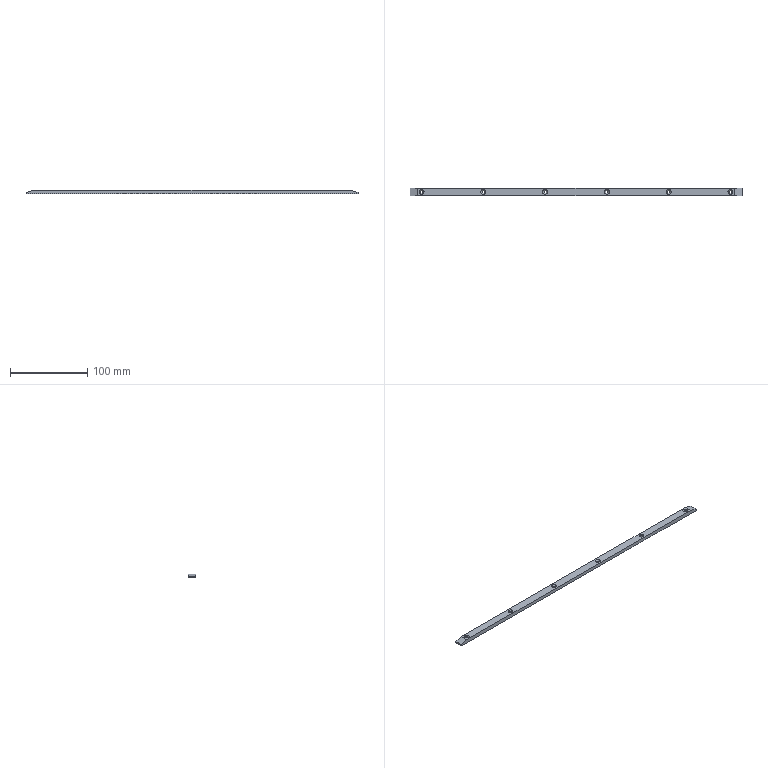Part | NX | features BREP 1 | 1 solid | 32 faces | box 430 x 10 x 5 mm | volume 20841 mm3 | cone 12 | cylinder 12 | plane 8 | commonest cylinder face diameters 3.4 x12
STEP:
#1=CARTESIAN_POINT('',(-203.15,0.,5.));
#2=VERTEX_POINT('',#1);
#3=CARTESIAN_POINT('',(-201.7,0.,3.55));
#4=VERTEX_POINT('',#3);
#5=CARTESIAN_POINT('',(-203.15,0.,5.));
#6=DIRECTION('',(-0.7071,0.,0.7071));
#7=VECTOR('',#6,1000.);
#8=LINE('',#5,#7);
#9=EDGE_CURVE('',#2,#4,#8,.F.);
#10=ORIENTED_EDGE('',*,*,#9,.T.);
#11=CARTESIAN_POINT('',(-198.3,0.,3.55));
#12=VERTEX_POINT('',#11);
#13=CARTESIAN_POINT('',(-200.,0.,3.55));
#14=DIRECTION('',(0.,0.,1.));
#15=DIRECTION('',(1.,0.,0.));
#16=AXIS2_PLACEMENT_3D('',#13,#14,#15);
#17=CIRCLE('',#16,1.7);
#18=EDGE_CURVE('',#12,#4,#17,.T.);
#19=ORIENTED_EDGE('',*,*,#18,.F.);
#20=CARTESIAN_POINT('',(-196.85,0.,5.));
#21=VERTEX_POINT('',#20);
#22=CARTESIAN_POINT('',(-196.85,0.,5.));
#23=DIRECTION('',(0.7071,0.,0.7071));
#24=VECTOR('',#23,1000.);
#25=LINE('',#22,#24);
#26=EDGE_CURVE('',#21,#12,#25,.F.);
#27=ORIENTED_EDGE('',*,*,#26,.F.);
#28=CARTESIAN_POINT('',(-200.,0.,5.));
#29=DIRECTION('',(0.,0.,1.));
#30=DIRECTION('',(1.,0.,0.));
#31=AXIS2_PLACEMENT_3D('',#28,#29,#30);
#32=CIRCLE('',#31,3.15);
#33=EDGE_CURVE('',#21,#2,#32,.T.);
#34=ORIENTED_EDGE('',*,*,#33,.T.);
#35=EDGE_LOOP('',(#10,#19,#27,#34));
#36=FACE_BOUND('',#35,.T.);
#37=CARTESIAN_POINT('',(-200.,0.,5.));
#38=DIRECTION('',(0.,0.,1.));
#39=DIRECTION('',(1.,0.,0.));
#40=AXIS2_PLACEMENT_3D('',#37,#38,#39);
#41=CONICAL_SURFACE('',#40,3.15,0.7854);
#42=ADVANCED_FACE('',(#36),#41,.F.);
#43=CARTESIAN_POINT('',(-201.7,0.,0.));
#44=VERTEX_POINT('',#43);
#45=CARTESIAN_POINT('',(-201.7,0.,5.));
#46=DIRECTION('',(0.,0.,1.));
#47=VECTOR('',#46,1000.);
#48=LINE('',#45,#47);
#49=EDGE_CURVE('',#4,#44,#48,.F.);
#50=ORIENTED_EDGE('',*,*,#49,.T.);
#51=CARTESIAN_POINT('',(-198.3,0.,0.));
#52=VERTEX_POINT('',#51);
#53=CARTESIAN_POINT('',(-200.,0.,0.));
#54=DIRECTION('',(0.,0.,1.));
#55=DIRECTION('',(1.,0.,0.));
#56=AXIS2_PLACEMENT_3D('',#53,#54,#55);
#57=CIRCLE('',#56,1.7);
#58=EDGE_CURVE('',#52,#44,#57,.T.);
#59=ORIENTED_EDGE('',*,*,#58,.F.);
#60=CARTESIAN_POINT('',(-198.3,0.,5.));
#61=DIRECTION('',(0.,0.,1.));
#62=VECTOR('',#61,1000.);
#63=LINE('',#60,#62);
#64=EDGE_CURVE('',#12,#52,#63,.F.);
#65=ORIENTED_EDGE('',*,*,#64,.F.);
#66=ORIENTED_EDGE('',*,*,#18,.T.);
#67=EDGE_LOOP('',(#50,#59,#65,#66));
#68=FACE_BOUND('',#67,.T.);
#69=CARTESIAN_POINT('',(-200.,0.,5.));
#70=DIRECTION('',(0.,0.,1.));
#71=DIRECTION('',(1.,0.,0.));
#72=AXIS2_PLACEMENT_3D('',#69,#70,#71);
#73=CYLINDRICAL_SURFACE('',#72,1.7);
#74=ADVANCED_FACE('',(#68),#73,.F.);
#75=CARTESIAN_POINT('',(-123.15,0.,5.));
#76=VERTEX_POINT('',#75);
#77=CARTESIAN_POINT('',(-121.7,0.,3.55));
#78=VERTEX_POINT('',#77);
#79=CARTESIAN_POINT('',(-123.15,0.,5.));
#80=DIRECTION('',(-0.7071,0.,0.7071));
#81=VECTOR('',#80,1000.);
#82=LINE('',#79,#81);
#83=EDGE_CURVE('',#76,#78,#82,.F.);
#84=ORIENTED_EDGE('',*,*,#83,.T.);
#85=CARTESIAN_POINT('',(-118.3,0.,3.55));
#86=VERTEX_POINT('',#85);
#87=CARTESIAN_POINT('',(-120.,0.,3.55));
#88=DIRECTION('',(0.,0.,1.));
#89=DIRECTION('',(1.,0.,0.));
#90=AXIS2_PLACEMENT_3D('',#87,#88,#89);
#91=CIRCLE('',#90,1.7);
#92=EDGE_CURVE('',#86,#78,#91,.T.);
#93=ORIENTED_EDGE('',*,*,#92,.F.);
#94=CARTESIAN_POINT('',(-116.85,0.,5.));
#95=VERTEX_POINT('',#94);
#96=CARTESIAN_POINT('',(-116.85,0.,5.));
#97=DIRECTION('',(0.7071,0.,0.7071));
#98=VECTOR('',#97,1000.);
#99=LINE('',#96,#98);
#100=EDGE_CURVE('',#95,#86,#99,.F.);
#101=ORIENTED_EDGE('',*,*,#100,.F.);
#102=CARTESIAN_POINT('',(-120.,0.,5.));
#103=DIRECTION('',(0.,0.,1.));
#104=DIRECTION('',(1.,0.,0.));
#105=AXIS2_PLACEMENT_3D('',#102,#103,#104);
#106=CIRCLE('',#105,3.15);
#107=EDGE_CURVE('',#95,#76,#106,.T.);
#108=ORIENTED_EDGE('',*,*,#107,.T.);
#109=EDGE_LOOP('',(#84,#93,#101,#108));
#110=FACE_BOUND('',#109,.T.);
#111=CARTESIAN_POINT('',(-120.,0.,5.));
#112=DIRECTION('',(0.,0.,1.));
#113=DIRECTION('',(1.,0.,0.));
#114=AXIS2_PLACEMENT_3D('',#111,#112,#113);
#115=CONICAL_SURFACE('',#114,3.15,0.7854);
#116=ADVANCED_FACE('',(#110),#115,.F.);
#117=CARTESIAN_POINT('',(-121.7,0.,0.));
#118=VERTEX_POINT('',#117);
#119=CARTESIAN_POINT('',(-121.7,0.,5.));
#120=DIRECTION('',(0.,0.,1.));
#121=VECTOR('',#120,1000.);
#122=LINE('',#119,#121);
#123=EDGE_CURVE('',#78,#118,#122,.F.);
#124=ORIENTED_EDGE('',*,*,#123,.T.);
#125=CARTESIAN_POINT('',(-118.3,0.,0.));
#126=VERTEX_POINT('',#125);
#127=CARTESIAN_POINT('',(-120.,0.,0.));
#128=DIRECTION('',(0.,0.,1.));
#129=DIRECTION('',(1.,0.,0.));
#130=AXIS2_PLACEMENT_3D('',#127,#128,#129);
#131=CIRCLE('',#130,1.7);
#132=EDGE_CURVE('',#126,#118,#131,.T.);
#133=ORIENTED_EDGE('',*,*,#132,.F.);
#134=CARTESIAN_POINT('',(-118.3,0.,5.));
#135=DIRECTION('',(0.,0.,1.));
#136=VECTOR('',#135,1000.);
#137=LINE('',#134,#136);
#138=EDGE_CURVE('',#86,#126,#137,.F.);
#139=ORIENTED_EDGE('',*,*,#138,.F.);
#140=ORIENTED_EDGE('',*,*,#92,.T.);
#141=EDGE_LOOP('',(#124,#133,#139,#140));
#142=FACE_BOUND('',#141,.T.);
#143=CARTESIAN_POINT('',(-120.,0.,5.));
#144=DIRECTION('',(0.,0.,1.));
#145=DIRECTION('',(1.,0.,0.));
#146=AXIS2_PLACEMENT_3D('',#143,#144,#145);
#147=CYLINDRICAL_SURFACE('',#146,1.7);
#148=ADVANCED_FACE('',(#142),#147,.F.);
#149=CARTESIAN_POINT('',(-43.15,0.,5.));
#150=VERTEX_POINT('',#149);
#151=CARTESIAN_POINT('',(-41.7,0.,3.55));
#152=VERTEX_POINT('',#151);
#153=CARTESIAN_POINT('',(-43.15,0.,5.));
#154=DIRECTION('',(-0.7071,0.,0.7071));
#155=VECTOR('',#154,1000.);
#156=LINE('',#153,#155);
#157=EDGE_CURVE('',#150,#152,#156,.F.);
#158=ORIENTED_EDGE('',*,*,#157,.T.);
#159=CARTESIAN_POINT('',(-38.3,0.,3.55));
#160=VERTEX_POINT('',#159);
#161=CARTESIAN_POINT('',(-40.,0.,3.55));
#162=DIRECTION('',(0.,0.,1.));
#163=DIRECTION('',(1.,0.,0.));
#164=AXIS2_PLACEMENT_3D('',#161,#162,#163);
#165=CIRCLE('',#164,1.7);
#166=EDGE_CURVE('',#160,#152,#165,.T.);
#167=ORIENTED_EDGE('',*,*,#166,.F.);
#168=CARTESIAN_POINT('',(-36.85,0.,5.));
#169=VERTEX_POINT('',#168);
#170=CARTESIAN_POINT('',(-36.85,0.,5.));
#171=DIRECTION('',(0.7071,0.,0.7071));
#172=VECTOR('',#171,1000.);
#173=LINE('',#170,#172);
#174=EDGE_CURVE('',#169,#160,#173,.F.);
#175=ORIENTED_EDGE('',*,*,#174,.F.);
#176=CARTESIAN_POINT('',(-40.,0.,5.));
#177=DIRECTION('',(0.,0.,1.));
#178=DIRECTION('',(1.,0.,0.));
#179=AXIS2_PLACEMENT_3D('',#176,#177,#178);
#180=CIRCLE('',#179,3.15);
#181=EDGE_CURVE('',#169,#150,#180,.T.);
#182=ORIENTED_EDGE('',*,*,#181,.T.);
#183=EDGE_LOOP('',(#158,#167,#175,#182));
#184=FACE_BOUND('',#183,.T.);
#185=CARTESIAN_POINT('',(-40.,0.,5.));
#186=DIRECTION('',(0.,0.,1.));
#187=DIRECTION('',(1.,0.,0.));
#188=AXIS2_PLACEMENT_3D('',#185,#186,#187);
#189=CONICAL_SURFACE('',#188,3.15,0.7854);
#190=ADVANCED_FACE('',(#184),#189,.F.);
#191=CARTESIAN_POINT('',(-41.7,0.,0.));
#192=VERTEX_POINT('',#191);
#193=CARTESIAN_POINT('',(-41.7,0.,5.));
#194=DIRECTION('',(0.,0.,1.));
#195=VECTOR('',#194,1000.);
#196=LINE('',#193,#195);
#197=EDGE_CURVE('',#152,#192,#196,.F.);
#198=ORIENTED_EDGE('',*,*,#197,.T.);
#199=CARTESIAN_POINT('',(-38.3,0.,0.));
#200=VERTEX_POINT('',#199);
#201=CARTESIAN_POINT('',(-40.,0.,0.));
#202=DIRECTION('',(0.,0.,1.));
#203=DIRECTION('',(1.,0.,0.));
#204=AXIS2_PLACEMENT_3D('',#201,#202,#203);
#205=CIRCLE('',#204,1.7);
#206=EDGE_CURVE('',#200,#192,#205,.T.);
#207=ORIENTED_EDGE('',*,*,#206,.F.);
#208=CARTESIAN_POINT('',(-38.3,0.,5.));
#209=DIRECTION('',(0.,0.,1.));
#210=VECTOR('',#209,1000.);
#211=LINE('',#208,#210);
#212=EDGE_CURVE('',#160,#200,#211,.F.);
#213=ORIENTED_EDGE('',*,*,#212,.F.);
#214=ORIENTED_EDGE('',*,*,#166,.T.);
#215=EDGE_LOOP('',(#198,#207,#213,#214));
#216=FACE_BOUND('',#215,.T.);
#217=CARTESIAN_POINT('',(-40.,0.,5.));
#218=DIRECTION('',(0.,0.,1.));
#219=DIRECTION('',(1.,0.,0.));
#220=AXIS2_PLACEMENT_3D('',#217,#218,#219);
#221=CYLINDRICAL_SURFACE('',#220,1.7);
#222=ADVANCED_FACE('',(#216),#221,.F.);
#223=CARTESIAN_POINT('',(36.85,0.,5.));
#224=VERTEX_POINT('',#223);
#225=CARTESIAN_POINT('',(38.3,0.,3.55));
#226=VERTEX_POINT('',#225);
#227=CARTESIAN_POINT('',(36.85,0.,5.));
#228=DIRECTION('',(-0.7071,0.,0.7071));
#229=VECTOR('',#228,1000.);
#230=LINE('',#227,#229);
#231=EDGE_CURVE('',#224,#226,#230,.F.);
#232=ORIENTED_EDGE('',*,*,#231,.T.);
#233=CARTESIAN_POINT('',(41.7,0.,3.55));
#234=VERTEX_POINT('',#233);
#235=CARTESIAN_POINT('',(40.,0.,3.55));
#236=DIRECTION('',(0.,0.,1.));
#237=DIRECTION('',(1.,0.,0.));
#238=AXIS2_PLACEMENT_3D('',#235,#236,#237);
#239=CIRCLE('',#238,1.7);
#240=EDGE_CURVE('',#234,#226,#239,.T.);
#241=ORIENTED_EDGE('',*,*,#240,.F.);
#242=CARTESIAN_POINT('',(43.15,0.,5.));
#243=VERTEX_POINT('',#242);
#244=CARTESIAN_POINT('',(43.15,0.,5.));
#245=DIRECTION('',(0.7071,0.,0.7071));
#246=VECTOR('',#245,1000.);
#247=LINE('',#244,#246);
#248=EDGE_CURVE('',#243,#234,#247,.F.);
#249=ORIENTED_EDGE('',*,*,#248,.F.);
#250=CARTESIAN_POINT('',(40.,0.,5.));
#251=DIRECTION('',(0.,0.,1.));
#252=DIRECTION('',(1.,0.,0.));
#253=AXIS2_PLACEMENT_3D('',#250,#251,#252);
#254=CIRCLE('',#253,3.15);
#255=EDGE_CURVE('',#243,#224,#254,.T.);
#256=ORIENTED_EDGE('',*,*,#255,.T.);
#257=EDGE_LOOP('',(#232,#241,#249,#256));
#258=FACE_BOUND('',#257,.T.);
#259=CARTESIAN_POINT('',(40.,0.,5.));
#260=DIRECTION('',(0.,0.,1.));
#261=DIRECTION('',(1.,0.,0.));
#262=AXIS2_PLACEMENT_3D('',#259,#260,#261);
#263=CONICAL_SURFACE('',#262,3.15,0.7854);
#264=ADVANCED_FACE('',(#258),#263,.F.);
#265=CARTESIAN_POINT('',(38.3,0.,0.));
#266=VERTEX_POINT('',#265);
#267=CARTESIAN_POINT('',(38.3,0.,5.));
#268=DIRECTION('',(0.,0.,1.));
#269=VECTOR('',#268,1000.);
#270=LINE('',#267,#269);
#271=EDGE_CURVE('',#226,#266,#270,.F.);
#272=ORIENTED_EDGE('',*,*,#271,.T.);
#273=CARTESIAN_POINT('',(41.7,0.,0.));
#274=VERTEX_POINT('',#273);
#275=CARTESIAN_POINT('',(40.,0.,0.));
#276=DIRECTION('',(0.,0.,1.));
#277=DIRECTION('',(1.,0.,0.));
#278=AXIS2_PLACEMENT_3D('',#275,#276,#277);
#279=CIRCLE('',#278,1.7);
#280=EDGE_CURVE('',#274,#266,#279,.T.);
#281=ORIENTED_EDGE('',*,*,#280,.F.);
#282=CARTESIAN_POINT('',(41.7,0.,5.));
#283=DIRECTION('',(0.,0.,1.));
#284=VECTOR('',#283,1000.);
#285=LINE('',#282,#284);
#286=EDGE_CURVE('',#234,#274,#285,.F.);
#287=ORIENTED_EDGE('',*,*,#286,.F.);
#288=ORIENTED_EDGE('',*,*,#240,.T.);
#289=EDGE_LOOP('',(#272,#281,#287,#288));
#290=FACE_BOUND('',#289,.T.);
#291=CARTESIAN_POINT('',(40.,0.,5.));
#292=DIRECTION('',(0.,0.,1.));
#293=DIRECTION('',(1.,0.,0.));
#294=AXIS2_PLACEMENT_3D('',#291,#292,#293);
#295=CYLINDRICAL_SURFACE('',#294,1.7);
#296=ADVANCED_FACE('',(#290),#295,.F.);
#297=CARTESIAN_POINT('',(116.85,0.,5.));
#298=VERTEX_POINT('',#297);
#299=CARTESIAN_POINT('',(118.3,0.,3.55));
#300=VERTEX_POINT('',#299);
#301=CARTESIAN_POINT('',(116.85,0.,5.));
#302=DIRECTION('',(-0.7071,0.,0.7071));
#303=VECTOR('',#302,1000.);
#304=LINE('',#301,#303);
#305=EDGE_CURVE('',#298,#300,#304,.F.);
#306=ORIENTED_EDGE('',*,*,#305,.T.);
#307=CARTESIAN_POINT('',(121.7,0.,3.55));
#308=VERTEX_POINT('',#307);
#309=CARTESIAN_POINT('',(120.,0.,3.55));
#310=DIRECTION('',(0.,0.,1.));
#311=DIRECTION('',(1.,0.,0.));
#312=AXIS2_PLACEMENT_3D('',#309,#310,#311);
#313=CIRCLE('',#312,1.7);
#314=EDGE_CURVE('',#308,#300,#313,.T.);
#315=ORIENTED_EDGE('',*,*,#314,.F.);
#316=CARTESIAN_POINT('',(123.15,0.,5.));
#317=VERTEX_POINT('',#316);
#318=CARTESIAN_POINT('',(123.15,0.,5.));
#319=DIRECTION('',(0.7071,0.,0.7071));
#320=VECTOR('',#319,1000.);
#321=LINE('',#318,#320);
#322=EDGE_CURVE('',#317,#308,#321,.F.);
#323=ORIENTED_EDGE('',*,*,#322,.F.);
#324=CARTESIAN_POINT('',(120.,0.,5.));
#325=DIRECTION('',(0.,0.,1.));
#326=DIRECTION('',(1.,0.,0.));
#327=AXIS2_PLACEMENT_3D('',#324,#325,#326);
#328=CIRCLE('',#327,3.15);
#329=EDGE_CURVE('',#317,#298,#328,.T.);
#330=ORIENTED_EDGE('',*,*,#329,.T.);
#331=EDGE_LOOP('',(#306,#315,#323,#330));
#332=FACE_BOUND('',#331,.T.);
#333=CARTESIAN_POINT('',(120.,0.,5.));
#334=DIRECTION('',(0.,0.,1.));
#335=DIRECTION('',(1.,0.,0.));
#336=AXIS2_PLACEMENT_3D('',#333,#334,#335);
#337=CONICAL_SURFACE('',#336,3.15,0.7854);
#338=ADVANCED_FACE('',(#332),#337,.F.);
#339=CARTESIAN_POINT('',(118.3,0.,0.));
#340=VERTEX_POINT('',#339);
#341=CARTESIAN_POINT('',(118.3,0.,5.));
#342=DIRECTION('',(0.,0.,1.));
#343=VECTOR('',#342,1000.);
#344=LINE('',#341,#343);
#345=EDGE_CURVE('',#300,#340,#344,.F.);
#346=ORIENTED_EDGE('',*,*,#345,.T.);
#347=CARTESIAN_POINT('',(121.7,0.,0.));
#348=VERTEX_POINT('',#347);
#349=CARTESIAN_POINT('',(120.,0.,0.));
#350=DIRECTION('',(0.,0.,1.));
#351=DIRECTION('',(1.,0.,0.));
#352=AXIS2_PLACEMENT_3D('',#349,#350,#351);
#353=CIRCLE('',#352,1.7);
#354=EDGE_CURVE('',#348,#340,#353,.T.);
#355=ORIENTED_EDGE('',*,*,#354,.F.);
#356=CARTESIAN_POINT('',(121.7,0.,5.));
#357=DIRECTION('',(0.,0.,1.));
#358=VECTOR('',#357,1000.);
#359=LINE('',#356,#358);
#360=EDGE_CURVE('',#308,#348,#359,.F.);
#361=ORIENTED_EDGE('',*,*,#360,.F.);
#362=ORIENTED_EDGE('',*,*,#314,.T.);
#363=EDGE_LOOP('',(#346,#355,#361,#362));
#364=FACE_BOUND('',#363,.T.);
#365=CARTESIAN_POINT('',(120.,0.,5.));
#366=DIRECTION('',(0.,0.,1.));
#367=DIRECTION('',(1.,0.,0.));
#368=AXIS2_PLACEMENT_3D('',#365,#366,#367);
#369=CYLINDRICAL_SURFACE('',#368,1.7);
#370=ADVANCED_FACE('',(#364),#369,.F.);
#371=CARTESIAN_POINT('',(196.85,0.,5.));
#372=VERTEX_POINT('',#371);
#373=CARTESIAN_POINT('',(198.3,0.,3.55));
#374=VERTEX_POINT('',#373);
#375=CARTESIAN_POINT('',(196.85,0.,5.));
#376=DIRECTION('',(-0.7071,0.,0.7071));
#377=VECTOR('',#376,1000.);
#378=LINE('',#375,#377);
#379=EDGE_CURVE('',#372,#374,#378,.F.);
#380=ORIENTED_EDGE('',*,*,#379,.T.);
#381=CARTESIAN_POINT('',(201.7,0.,3.55));
#382=VERTEX_POINT('',#381);
#383=CARTESIAN_POINT('',(200.,0.,3.55));
#384=DIRECTION('',(0.,0.,1.));
#385=DIRECTION('',(1.,0.,0.));
#386=AXIS2_PLACEMENT_3D('',#383,#384,#385);
#387=CIRCLE('',#386,1.7);
#388=EDGE_CURVE('',#382,#374,#387,.T.);
#389=ORIENTED_EDGE('',*,*,#388,.F.);
#390=CARTESIAN_POINT('',(203.15,0.,5.));
#391=VERTEX_POINT('',#390);
#392=CARTESIAN_POINT('',(203.15,0.,5.));
#393=DIRECTION('',(0.7071,0.,0.7071));
#394=VECTOR('',#393,1000.);
#395=LINE('',#392,#394);
#396=EDGE_CURVE('',#391,#382,#395,.F.);
#397=ORIENTED_EDGE('',*,*,#396,.F.);
#398=CARTESIAN_POINT('',(200.,0.,5.));
#399=DIRECTION('',(0.,0.,1.));
#400=DIRECTION('',(1.,0.,0.));
#401=AXIS2_PLACEMENT_3D('',#398,#399,#400);
#402=CIRCLE('',#401,3.15);
#403=EDGE_CURVE('',#391,#372,#402,.T.);
#404=ORIENTED_EDGE('',*,*,#403,.T.);
#405=EDGE_LOOP('',(#380,#389,#397,#404));
#406=FACE_BOUND('',#405,.T.);
#407=CARTESIAN_POINT('',(200.,0.,5.));
#408=DIRECTION('',(0.,0.,1.));
#409=DIRECTION('',(1.,0.,0.));
#410=AXIS2_PLACEMENT_3D('',#407,#408,#409);
#411=CONICAL_SURFACE('',#410,3.15,0.7854);
#412=ADVANCED_FACE('',(#406),#411,.F.);
#413=CARTESIAN_POINT('',(198.3,0.,0.));
#414=VERTEX_POINT('',#413);
#415=CARTESIAN_POINT('',(198.3,0.,5.));
#416=DIRECTION('',(0.,0.,1.));
#417=VECTOR('',#416,1000.);
#418=LINE('',#415,#417);
#419=EDGE_CURVE('',#374,#414,#418,.F.);
#420=ORIENTED_EDGE('',*,*,#419,.T.);
#421=CARTESIAN_POINT('',(201.7,0.,0.));
#422=VERTEX_POINT('',#421);
#423=CARTESIAN_POINT('',(200.,0.,0.));
#424=DIRECTION('',(0.,0.,1.));
#425=DIRECTION('',(1.,0.,0.));
#426=AXIS2_PLACEMENT_3D('',#423,#424,#425);
#427=CIRCLE('',#426,1.7);
#428=EDGE_CURVE('',#422,#414,#427,.T.);
#429=ORIENTED_EDGE('',*,*,#428,.F.);
#430=CARTESIAN_POINT('',(201.7,0.,5.));
#431=DIRECTION('',(0.,0.,1.));
#432=VECTOR('',#431,1000.);
#433=LINE('',#430,#432);
#434=EDGE_CURVE('',#382,#422,#433,.F.);
#435=ORIENTED_EDGE('',*,*,#434,.F.);
#436=ORIENTED_EDGE('',*,*,#388,.T.);
#437=EDGE_LOOP('',(#420,#429,#435,#436));
#438=FACE_BOUND('',#437,.T.);
#439=CARTESIAN_POINT('',(200.,0.,5.));
#440=DIRECTION('',(0.,0.,1.));
#441=DIRECTION('',(1.,0.,0.));
#442=AXIS2_PLACEMENT_3D('',#439,#440,#441);
#443=CYLINDRICAL_SURFACE('',#442,1.7);
#444=ADVANCED_FACE('',(#438),#443,.F.);
#445=CARTESIAN_POINT('',(-215.,5.,2.));
#446=VERTEX_POINT('',#445);
#447=CARTESIAN_POINT('',(-205.,5.,5.));
#448=VERTEX_POINT('',#447);
#449=CARTESIAN_POINT('',(-205.,5.,5.));
#450=DIRECTION('',(0.9578,0.,0.2873));
#451=VECTOR('',#450,1000.);
#452=LINE('',#449,#451);
#453=EDGE_CURVE('',#446,#448,#452,.T.);
#454=ORIENTED_EDGE('',*,*,#453,.F.);
#455=CARTESIAN_POINT('',(-215.,-5.,2.));
#456=VERTEX_POINT('',#455);
#457=CARTESIAN_POINT('',(-215.,-5.,2.));
#458=DIRECTION('',(0.,1.,0.));
#459=VECTOR('',#458,1000.);
#460=LINE('',#457,#459);
#461=EDGE_CURVE('',#456,#446,#460,.T.);
#462=ORIENTED_EDGE('',*,*,#461,.F.);
#463=CARTESIAN_POINT('',(-205.,-5.,5.));
#464=VERTEX_POINT('',#463);
#465=CARTESIAN_POINT('',(-205.,-5.,5.));
#466=DIRECTION('',(-0.9578,0.,-0.2873));
#467=VECTOR('',#466,1000.);
#468=LINE('',#465,#467);
#469=EDGE_CURVE('',#464,#456,#468,.T.);
#470=ORIENTED_EDGE('',*,*,#469,.F.);
#471=CARTESIAN_POINT('',(-205.,0.,5.));
#472=DIRECTION('',(0.,-1.,0.));
#473=VECTOR('',#472,1000.);
#474=LINE('',#471,#473);
#475=EDGE_CURVE('',#448,#464,#474,.T.);
#476=ORIENTED_EDGE('',*,*,#475,.F.);
#477=EDGE_LOOP('',(#454,#462,#470,#476));
#478=FACE_BOUND('',#477,.T.);
#479=CARTESIAN_POINT('',(-205.,0.,5.));
#480=DIRECTION('',(0.2873,0.,-0.9578));
#481=DIRECTION('',(0.,-1.,0.));
#482=AXIS2_PLACEMENT_3D('',#479,#480,#481);
#483=PLANE('',#482);
#484=ADVANCED_FACE('',(#478),#483,.F.);
#485=CARTESIAN_POINT('',(215.,-5.,2.));
#486=VERTEX_POINT('',#485);
#487=CARTESIAN_POINT('',(205.,-5.,5.));
#488=VERTEX_POINT('',#487);
#489=CARTESIAN_POINT('',(205.,-5.,5.));
#490=DIRECTION('',(-0.9578,0.,0.2873));
#491=VECTOR('',#490,1000.);
#492=LINE('',#489,#491);
#493=EDGE_CURVE('',#486,#488,#492,.T.);
#494=ORIENTED_EDGE('',*,*,#493,.F.);
#495=CARTESIAN_POINT('',(215.,5.,2.));
#496=VERTEX_POINT('',#495);
#497=CARTESIAN_POINT('',(215.,-5.,2.));
#498=DIRECTION('',(0.,-1.,0.));
#499=VECTOR('',#498,1000.);
#500=LINE('',#497,#499);
#501=EDGE_CURVE('',#496,#486,#500,.T.);
#502=ORIENTED_EDGE('',*,*,#501,.F.);
#503=CARTESIAN_POINT('',(205.,5.,5.));
#504=VERTEX_POINT('',#503);
#505=CARTESIAN_POINT('',(205.,5.,5.));
#506=DIRECTION('',(0.9578,0.,-0.2873));
#507=VECTOR('',#506,1000.);
#508=LINE('',#505,#507);
#509=EDGE_CURVE('',#504,#496,#508,.T.);
#510=ORIENTED_EDGE('',*,*,#509,.F.);
#511=CARTESIAN_POINT('',(205.,0.,5.));
#512=DIRECTION('',(0.,1.,0.));
#513=VECTOR('',#512,1000.);
#514=LINE('',#511,#513);
#515=EDGE_CURVE('',#488,#504,#514,.T.);
#516=ORIENTED_EDGE('',*,*,#515,.F.);
#517=EDGE_LOOP('',(#494,#502,#510,#516));
#518=FACE_BOUND('',#517,.T.);
#519=CARTESIAN_POINT('',(205.,0.,5.));
#520=DIRECTION('',(-0.2873,0.,-0.9578));
#521=DIRECTION('',(0.,1.,0.));
#522=AXIS2_PLACEMENT_3D('',#519,#520,#521);
#523=PLANE('',#522);
#524=ADVANCED_FACE('',(#518),#523,.F.);
#525=CARTESIAN_POINT('',(215.,-5.,0.));
#526=VERTEX_POINT('',#525);
#527=CARTESIAN_POINT('',(215.,5.,0.));
#528=VERTEX_POINT('',#527);
#529=CARTESIAN_POINT('',(215.,-5.,0.));
#530=DIRECTION('',(0.,1.,0.));
#531=VECTOR('',#530,1000.);
#532=LINE('',#529,#531);
#533=EDGE_CURVE('',#526,#528,#532,.T.);
#534=ORIENTED_EDGE('',*,*,#533,.F.);
#535=CARTESIAN_POINT('',(-215.,-5.,0.));
#536=VERTEX_POINT('',#535);
#537=CARTESIAN_POINT('',(-215.,-5.,0.));
#538=DIRECTION('',(1.,0.,0.));
#539=VECTOR('',#538,1000.);
#540=LINE('',#537,#539);
#541=EDGE_CURVE('',#536,#526,#540,.T.);
#542=ORIENTED_EDGE('',*,*,#541,.F.);
#543=CARTESIAN_POINT('',(-215.,5.,0.));
#544=VERTEX_POINT('',#543);
#545=CARTESIAN_POINT('',(-215.,-5.,0.));
#546=DIRECTION('',(0.,-1.,0.));
#547=VECTOR('',#546,1000.);
#548=LINE('',#545,#547);
#549=EDGE_CURVE('',#544,#536,#548,.T.);
#550=ORIENTED_EDGE('',*,*,#549,.F.);
#551=CARTESIAN_POINT('',(-215.,5.,0.));
#552=DIRECTION('',(-1.,0.,0.));
#553=VECTOR('',#552,1000.);
#554=LINE('',#551,#553);
#555=EDGE_CURVE('',#528,#544,#554,.T.);
#556=ORIENTED_EDGE('',*,*,#555,.F.);
#557=EDGE_LOOP('',(#534,#542,#550,#556));
#558=FACE_BOUND('',#557,.T.);
#559=ORIENTED_EDGE('',*,*,#428,.T.);
#560=CARTESIAN_POINT('',(200.,0.,0.));
#561=DIRECTION('',(0.,0.,1.));
#562=DIRECTION('',(1.,0.,0.));
#563=AXIS2_PLACEMENT_3D('',#560,#561,#562);
#564=CIRCLE('',#563,1.7);
#565=EDGE_CURVE('',#414,#422,#564,.T.);
#566=ORIENTED_EDGE('',*,*,#565,.T.);
#567=EDGE_LOOP('',(#559,#566));
#568=FACE_BOUND('',#567,.T.);
#569=ORIENTED_EDGE('',*,*,#354,.T.);
#570=CARTESIAN_POINT('',(120.,0.,0.));
#571=DIRECTION('',(0.,0.,1.));
#572=DIRECTION('',(1.,0.,0.));
#573=AXIS2_PLACEMENT_3D('',#570,#571,#572);
#574=CIRCLE('',#573,1.7);
#575=EDGE_CURVE('',#340,#348,#574,.T.);
#576=ORIENTED_EDGE('',*,*,#575,.T.);
#577=EDGE_LOOP('',(#569,#576));
#578=FACE_BOUND('',#577,.T.);
#579=ORIENTED_EDGE('',*,*,#280,.T.);
#580=CARTESIAN_POINT('',(40.,0.,0.));
#581=DIRECTION('',(0.,0.,1.));
#582=DIRECTION('',(1.,0.,0.));
#583=AXIS2_PLACEMENT_3D('',#580,#581,#582);
#584=CIRCLE('',#583,1.7);
#585=EDGE_CURVE('',#266,#274,#584,.T.);
#586=ORIENTED_EDGE('',*,*,#585,.T.);
#587=EDGE_LOOP('',(#579,#586));
#588=FACE_BOUND('',#587,.T.);
#589=ORIENTED_EDGE('',*,*,#206,.T.);
#590=CARTESIAN_POINT('',(-40.,0.,0.));
#591=DIRECTION('',(0.,0.,1.));
#592=DIRECTION('',(1.,0.,0.));
#593=AXIS2_PLACEMENT_3D('',#590,#591,#592);
#594=CIRCLE('',#593,1.7);
#595=EDGE_CURVE('',#192,#200,#594,.T.);
#596=ORIENTED_EDGE('',*,*,#595,.T.);
#597=EDGE_LOOP('',(#589,#596));
#598=FACE_BOUND('',#597,.T.);
#599=ORIENTED_EDGE('',*,*,#132,.T.);
#600=CARTESIAN_POINT('',(-120.,0.,0.));
#601=DIRECTION('',(0.,0.,1.));
#602=DIRECTION('',(1.,0.,0.));
#603=AXIS2_PLACEMENT_3D('',#600,#601,#602);
#604=CIRCLE('',#603,1.7);
#605=EDGE_CURVE('',#118,#126,#604,.T.);
#606=ORIENTED_EDGE('',*,*,#605,.T.);
#607=EDGE_LOOP('',(#599,#606));
#608=FACE_BOUND('',#607,.T.);
#609=ORIENTED_EDGE('',*,*,#58,.T.);
#610=CARTESIAN_POINT('',(-200.,0.,0.));
#611=DIRECTION('',(0.,0.,1.));
#612=DIRECTION('',(1.,0.,0.));
#613=AXIS2_PLACEMENT_3D('',#610,#611,#612);
#614=CIRCLE('',#613,1.7);
#615=EDGE_CURVE('',#44,#52,#614,.T.);
#616=ORIENTED_EDGE('',*,*,#615,.T.);
#617=EDGE_LOOP('',(#609,#616));
#618=FACE_BOUND('',#617,.T.);
#619=CARTESIAN_POINT('',(0.,0.,0.));
#620=DIRECTION('',(0.,0.,-1.));
#621=DIRECTION('',(-1.,0.,0.));
#622=AXIS2_PLACEMENT_3D('',#619,#620,#621);
#623=PLANE('',#622);
#624=ADVANCED_FACE('',(#558,#568,#578,#588,#598,#608,#618),#623,.T.);
#625=CARTESIAN_POINT('',(215.,-5.,5.));
#626=DIRECTION('',(0.,0.,-1.));
#627=VECTOR('',#626,1000.);
#628=LINE('',#625,#627);
#629=EDGE_CURVE('',#486,#526,#628,.T.);
#630=ORIENTED_EDGE('',*,*,#629,.F.);
#631=ORIENTED_EDGE('',*,*,#493,.T.);
#632=CARTESIAN_POINT('',(-215.,-5.,5.));
#633=DIRECTION('',(1.,0.,0.));
#634=VECTOR('',#633,1000.);
#635=LINE('',#632,#634);
#636=EDGE_CURVE('',#464,#488,#635,.T.);
#637=ORIENTED_EDGE('',*,*,#636,.F.);
#638=ORIENTED_EDGE('',*,*,#469,.T.);
#639=CARTESIAN_POINT('',(-215.,-5.,5.));
#640=DIRECTION('',(0.,0.,-1.));
#641=VECTOR('',#640,1000.);
#642=LINE('',#639,#641);
#643=EDGE_CURVE('',#456,#536,#642,.T.);
#644=ORIENTED_EDGE('',*,*,#643,.T.);
#645=ORIENTED_EDGE('',*,*,#541,.T.);
#646=EDGE_LOOP('',(#630,#631,#637,#638,#644,#645));
#647=FACE_BOUND('',#646,.T.);
#648=CARTESIAN_POINT('',(-215.,-5.,5.));
#649=DIRECTION('',(0.,1.,0.));
#650=DIRECTION('',(0.,0.,1.));
#651=AXIS2_PLACEMENT_3D('',#648,#649,#650);
#652=PLANE('',#651);
#653=ADVANCED_FACE('',(#647),#652,.F.);
#654=ORIENTED_EDGE('',*,*,#643,.F.);
#655=ORIENTED_EDGE('',*,*,#461,.T.);
#656=CARTESIAN_POINT('',(-215.,5.,5.));
#657=DIRECTION('',(0.,0.,-1.));
#658=VECTOR('',#657,1000.);
#659=LINE('',#656,#658);
#660=EDGE_CURVE('',#446,#544,#659,.T.);
#661=ORIENTED_EDGE('',*,*,#660,.T.);
#662=ORIENTED_EDGE('',*,*,#549,.T.);
#663=EDGE_LOOP('',(#654,#655,#661,#662));
#664=FACE_BOUND('',#663,.T.);
#665=CARTESIAN_POINT('',(-215.,-5.,5.));
#666=DIRECTION('',(1.,0.,0.));
#667=DIRECTION('',(0.,0.,-1.));
#668=AXIS2_PLACEMENT_3D('',#665,#666,#667);
#669=PLANE('',#668);
#670=ADVANCED_FACE('',(#664),#669,.F.);
#671=CARTESIAN_POINT('',(-215.,5.,5.));
#672=DIRECTION('',(-1.,0.,0.));
#673=VECTOR('',#672,1000.);
#674=LINE('',#671,#673);
#675=EDGE_CURVE('',#504,#448,#674,.T.);
#676=ORIENTED_EDGE('',*,*,#675,.F.);
#677=ORIENTED_EDGE('',*,*,#509,.T.);
#678=CARTESIAN_POINT('',(215.,5.,5.));
#679=DIRECTION('',(0.,0.,-1.));
#680=VECTOR('',#679,1000.);
#681=LINE('',#678,#680);
#682=EDGE_CURVE('',#496,#528,#681,.T.);
#683=ORIENTED_EDGE('',*,*,#682,.T.);
#684=ORIENTED_EDGE('',*,*,#555,.T.);
#685=ORIENTED_EDGE('',*,*,#660,.F.);
#686=ORIENTED_EDGE('',*,*,#453,.T.);
#687=EDGE_LOOP('',(#676,#677,#683,#684,#685,#686));
#688=FACE_BOUND('',#687,.T.);
#689=CARTESIAN_POINT('',(-215.,5.,5.));
#690=DIRECTION('',(0.,-1.,0.));
#691=DIRECTION('',(0.,0.,-1.));
#692=AXIS2_PLACEMENT_3D('',#689,#690,#691);
#693=PLANE('',#692);
#694=ADVANCED_FACE('',(#688),#693,.F.);
#695=ORIENTED_EDGE('',*,*,#682,.F.);
#696=ORIENTED_EDGE('',*,*,#501,.T.);
#697=ORIENTED_EDGE('',*,*,#629,.T.);
#698=ORIENTED_EDGE('',*,*,#533,.T.);
#699=EDGE_LOOP('',(#695,#696,#697,#698));
#700=FACE_BOUND('',#699,.T.);
#701=CARTESIAN_POINT('',(215.,-5.,5.));
#702=DIRECTION('',(-1.,0.,0.));
#703=DIRECTION('',(0.,0.,1.));
#704=AXIS2_PLACEMENT_3D('',#701,#702,#703);
#705=PLANE('',#704);
#706=ADVANCED_FACE('',(#700),#705,.F.);
#707=ORIENTED_EDGE('',*,*,#255,.F.);
#708=CARTESIAN_POINT('',(40.,0.,5.));
#709=DIRECTION('',(0.,0.,1.));
#710=DIRECTION('',(1.,0.,0.));
#711=AXIS2_PLACEMENT_3D('',#708,#709,#710);
#712=CIRCLE('',#711,3.15);
#713=EDGE_CURVE('',#224,#243,#712,.T.);
#714=ORIENTED_EDGE('',*,*,#713,.F.);
#715=EDGE_LOOP('',(#707,#714));
#716=FACE_BOUND('',#715,.T.);
#717=ORIENTED_EDGE('',*,*,#636,.T.);
#718=ORIENTED_EDGE('',*,*,#515,.T.);
#719=ORIENTED_EDGE('',*,*,#675,.T.);
#720=ORIENTED_EDGE('',*,*,#475,.T.);
#721=EDGE_LOOP('',(#717,#718,#719,#720));
#722=FACE_BOUND('',#721,.T.);
#723=ORIENTED_EDGE('',*,*,#403,.F.);
#724=CARTESIAN_POINT('',(200.,0.,5.));
#725=DIRECTION('',(0.,0.,1.));
#726=DIRECTION('',(1.,0.,0.));
#727=AXIS2_PLACEMENT_3D('',#724,#725,#726);
#728=CIRCLE('',#727,3.15);
#729=EDGE_CURVE('',#372,#391,#728,.T.);
#730=ORIENTED_EDGE('',*,*,#729,.F.);
#731=EDGE_LOOP('',(#723,#730));
#732=FACE_BOUND('',#731,.T.);
#733=ORIENTED_EDGE('',*,*,#329,.F.);
#734=CARTESIAN_POINT('',(120.,0.,5.));
#735=DIRECTION('',(0.,0.,1.));
#736=DIRECTION('',(1.,0.,0.));
#737=AXIS2_PLACEMENT_3D('',#734,#735,#736);
#738=CIRCLE('',#737,3.15);
#739=EDGE_CURVE('',#298,#317,#738,.T.);
#740=ORIENTED_EDGE('',*,*,#739,.F.);
#741=EDGE_LOOP('',(#733,#740));
#742=FACE_BOUND('',#741,.T.);
#743=ORIENTED_EDGE('',*,*,#181,.F.);
#744=CARTESIAN_POINT('',(-40.,0.,5.));
#745=DIRECTION('',(0.,0.,1.));
#746=DIRECTION('',(1.,0.,0.));
#747=AXIS2_PLACEMENT_3D('',#744,#745,#746);
#748=CIRCLE('',#747,3.15);
#749=EDGE_CURVE('',#150,#169,#748,.T.);
#750=ORIENTED_EDGE('',*,*,#749,.F.);
#751=EDGE_LOOP('',(#743,#750));
#752=FACE_BOUND('',#751,.T.);
#753=ORIENTED_EDGE('',*,*,#107,.F.);
#754=CARTESIAN_POINT('',(-120.,0.,5.));
#755=DIRECTION('',(0.,0.,1.));
#756=DIRECTION('',(1.,0.,0.));
#757=AXIS2_PLACEMENT_3D('',#754,#755,#756);
#758=CIRCLE('',#757,3.15);
#759=EDGE_CURVE('',#76,#95,#758,.T.);
#760=ORIENTED_EDGE('',*,*,#759,.F.);
#761=EDGE_LOOP('',(#753,#760));
#762=FACE_BOUND('',#761,.T.);
#763=ORIENTED_EDGE('',*,*,#33,.F.);
#764=CARTESIAN_POINT('',(-200.,0.,5.));
#765=DIRECTION('',(0.,0.,1.));
#766=DIRECTION('',(1.,0.,0.));
#767=AXIS2_PLACEMENT_3D('',#764,#765,#766);
#768=CIRCLE('',#767,3.15);
#769=EDGE_CURVE('',#2,#21,#768,.T.);
#770=ORIENTED_EDGE('',*,*,#769,.F.);
#771=EDGE_LOOP('',(#763,#770));
#772=FACE_BOUND('',#771,.T.);
#773=CARTESIAN_POINT('',(0.,0.,5.));
#774=DIRECTION('',(0.,0.,-1.));
#775=DIRECTION('',(-1.,0.,0.));
#776=AXIS2_PLACEMENT_3D('',#773,#774,#775);
#777=PLANE('',#776);
#778=ADVANCED_FACE('',(#716,#722,#732,#742,#752,#762,#772),#777,.F.);
#779=ORIENTED_EDGE('',*,*,#565,.F.);
#780=ORIENTED_EDGE('',*,*,#419,.F.);
#781=CARTESIAN_POINT('',(200.,0.,3.55));
#782=DIRECTION('',(0.,0.,1.));
#783=DIRECTION('',(1.,0.,0.));
#784=AXIS2_PLACEMENT_3D('',#781,#782,#783);
#785=CIRCLE('',#784,1.7);
#786=EDGE_CURVE('',#374,#382,#785,.T.);
#787=ORIENTED_EDGE('',*,*,#786,.T.);
#788=ORIENTED_EDGE('',*,*,#434,.T.);
#789=EDGE_LOOP('',(#779,#780,#787,#788));
#790=FACE_BOUND('',#789,.T.);
#791=CARTESIAN_POINT('',(200.,0.,5.));
#792=DIRECTION('',(0.,0.,1.));
#793=DIRECTION('',(1.,0.,0.));
#794=AXIS2_PLACEMENT_3D('',#791,#792,#793);
#795=CYLINDRICAL_SURFACE('',#794,1.7);
#796=ADVANCED_FACE('',(#790),#795,.F.);
#797=ORIENTED_EDGE('',*,*,#786,.F.);
#798=ORIENTED_EDGE('',*,*,#379,.F.);
#799=ORIENTED_EDGE('',*,*,#729,.T.);
#800=ORIENTED_EDGE('',*,*,#396,.T.);
#801=EDGE_LOOP('',(#797,#798,#799,#800));
#802=FACE_BOUND('',#801,.T.);
#803=CARTESIAN_POINT('',(200.,0.,5.));
#804=DIRECTION('',(0.,0.,1.));
#805=DIRECTION('',(1.,0.,0.));
#806=AXIS2_PLACEMENT_3D('',#803,#804,#805);
#807=CONICAL_SURFACE('',#806,3.15,0.7854);
#808=ADVANCED_FACE('',(#802),#807,.F.);
#809=ORIENTED_EDGE('',*,*,#575,.F.);
#810=ORIENTED_EDGE('',*,*,#345,.F.);
#811=CARTESIAN_POINT('',(120.,0.,3.55));
#812=DIRECTION('',(0.,0.,1.));
#813=DIRECTION('',(1.,0.,0.));
#814=AXIS2_PLACEMENT_3D('',#811,#812,#813);
#815=CIRCLE('',#814,1.7);
#816=EDGE_CURVE('',#300,#308,#815,.T.);
#817=ORIENTED_EDGE('',*,*,#816,.T.);
#818=ORIENTED_EDGE('',*,*,#360,.T.);
#819=EDGE_LOOP('',(#809,#810,#817,#818));
#820=FACE_BOUND('',#819,.T.);
#821=CARTESIAN_POINT('',(120.,0.,5.));
#822=DIRECTION('',(0.,0.,1.));
#823=DIRECTION('',(1.,0.,0.));
#824=AXIS2_PLACEMENT_3D('',#821,#822,#823);
#825=CYLINDRICAL_SURFACE('',#824,1.7);
#826=ADVANCED_FACE('',(#820),#825,.F.);
#827=ORIENTED_EDGE('',*,*,#816,.F.);
#828=ORIENTED_EDGE('',*,*,#305,.F.);
#829=ORIENTED_EDGE('',*,*,#739,.T.);
#830=ORIENTED_EDGE('',*,*,#322,.T.);
#831=EDGE_LOOP('',(#827,#828,#829,#830));
#832=FACE_BOUND('',#831,.T.);
#833=CARTESIAN_POINT('',(120.,0.,5.));
#834=DIRECTION('',(0.,0.,1.));
#835=DIRECTION('',(1.,0.,0.));
#836=AXIS2_PLACEMENT_3D('',#833,#834,#835);
#837=CONICAL_SURFACE('',#836,3.15,0.7854);
#838=ADVANCED_FACE('',(#832),#837,.F.);
#839=ORIENTED_EDGE('',*,*,#585,.F.);
#840=ORIENTED_EDGE('',*,*,#271,.F.);
#841=CARTESIAN_POINT('',(40.,0.,3.55));
#842=DIRECTION('',(0.,0.,1.));
#843=DIRECTION('',(1.,0.,0.));
#844=AXIS2_PLACEMENT_3D('',#841,#842,#843);
#845=CIRCLE('',#844,1.7);
#846=EDGE_CURVE('',#226,#234,#845,.T.);
#847=ORIENTED_EDGE('',*,*,#846,.T.);
#848=ORIENTED_EDGE('',*,*,#286,.T.);
#849=EDGE_LOOP('',(#839,#840,#847,#848));
#850=FACE_BOUND('',#849,.T.);
#851=CARTESIAN_POINT('',(40.,0.,5.));
#852=DIRECTION('',(0.,0.,1.));
#853=DIRECTION('',(1.,0.,0.));
#854=AXIS2_PLACEMENT_3D('',#851,#852,#853);
#855=CYLINDRICAL_SURFACE('',#854,1.7);
#856=ADVANCED_FACE('',(#850),#855,.F.);
#857=ORIENTED_EDGE('',*,*,#846,.F.);
#858=ORIENTED_EDGE('',*,*,#231,.F.);
#859=ORIENTED_EDGE('',*,*,#713,.T.);
#860=ORIENTED_EDGE('',*,*,#248,.T.);
#861=EDGE_LOOP('',(#857,#858,#859,#860));
#862=FACE_BOUND('',#861,.T.);
#863=CARTESIAN_POINT('',(40.,0.,5.));
#864=DIRECTION('',(0.,0.,1.));
#865=DIRECTION('',(1.,0.,0.));
#866=AXIS2_PLACEMENT_3D('',#863,#864,#865);
#867=CONICAL_SURFACE('',#866,3.15,0.7854);
#868=ADVANCED_FACE('',(#862),#867,.F.);
#869=ORIENTED_EDGE('',*,*,#595,.F.);
#870=ORIENTED_EDGE('',*,*,#197,.F.);
#871=CARTESIAN_POINT('',(-40.,0.,3.55));
#872=DIRECTION('',(0.,0.,1.));
#873=DIRECTION('',(1.,0.,0.));
#874=AXIS2_PLACEMENT_3D('',#871,#872,#873);
#875=CIRCLE('',#874,1.7);
#876=EDGE_CURVE('',#152,#160,#875,.T.);
#877=ORIENTED_EDGE('',*,*,#876,.T.);
#878=ORIENTED_EDGE('',*,*,#212,.T.);
#879=EDGE_LOOP('',(#869,#870,#877,#878));
#880=FACE_BOUND('',#879,.T.);
#881=CARTESIAN_POINT('',(-40.,0.,5.));
#882=DIRECTION('',(0.,0.,1.));
#883=DIRECTION('',(1.,0.,0.));
#884=AXIS2_PLACEMENT_3D('',#881,#882,#883);
#885=CYLINDRICAL_SURFACE('',#884,1.7);
#886=ADVANCED_FACE('',(#880),#885,.F.);
#887=ORIENTED_EDGE('',*,*,#876,.F.);
#888=ORIENTED_EDGE('',*,*,#157,.F.);
#889=ORIENTED_EDGE('',*,*,#749,.T.);
#890=ORIENTED_EDGE('',*,*,#174,.T.);
#891=EDGE_LOOP('',(#887,#888,#889,#890));
#892=FACE_BOUND('',#891,.T.);
#893=CARTESIAN_POINT('',(-40.,0.,5.));
#894=DIRECTION('',(0.,0.,1.));
#895=DIRECTION('',(1.,0.,0.));
#896=AXIS2_PLACEMENT_3D('',#893,#894,#895);
#897=CONICAL_SURFACE('',#896,3.15,0.7854);
#898=ADVANCED_FACE('',(#892),#897,.F.);
#899=ORIENTED_EDGE('',*,*,#605,.F.);
#900=ORIENTED_EDGE('',*,*,#123,.F.);
#901=CARTESIAN_POINT('',(-120.,0.,3.55));
#902=DIRECTION('',(0.,0.,1.));
#903=DIRECTION('',(1.,0.,0.));
#904=AXIS2_PLACEMENT_3D('',#901,#902,#903);
#905=CIRCLE('',#904,1.7);
#906=EDGE_CURVE('',#78,#86,#905,.T.);
#907=ORIENTED_EDGE('',*,*,#906,.T.);
#908=ORIENTED_EDGE('',*,*,#138,.T.);
#909=EDGE_LOOP('',(#899,#900,#907,#908));
#910=FACE_BOUND('',#909,.T.);
#911=CARTESIAN_POINT('',(-120.,0.,5.));
#912=DIRECTION('',(0.,0.,1.));
#913=DIRECTION('',(1.,0.,0.));
#914=AXIS2_PLACEMENT_3D('',#911,#912,#913);
#915=CYLINDRICAL_SURFACE('',#914,1.7);
#916=ADVANCED_FACE('',(#910),#915,.F.);
#917=ORIENTED_EDGE('',*,*,#906,.F.);
#918=ORIENTED_EDGE('',*,*,#83,.F.);
#919=ORIENTED_EDGE('',*,*,#759,.T.);
#920=ORIENTED_EDGE('',*,*,#100,.T.);
#921=EDGE_LOOP('',(#917,#918,#919,#920));
#922=FACE_BOUND('',#921,.T.);
#923=CARTESIAN_POINT('',(-120.,0.,5.));
#924=DIRECTION('',(0.,0.,1.));
#925=DIRECTION('',(1.,0.,0.));
#926=AXIS2_PLACEMENT_3D('',#923,#924,#925);
#927=CONICAL_SURFACE('',#926,3.15,0.7854);
#928=ADVANCED_FACE('',(#922),#927,.F.);
#929=ORIENTED_EDGE('',*,*,#615,.F.);
#930=ORIENTED_EDGE('',*,*,#49,.F.);
#931=CARTESIAN_POINT('',(-200.,0.,3.55));
#932=DIRECTION('',(0.,0.,1.));
#933=DIRECTION('',(1.,0.,0.));
#934=AXIS2_PLACEMENT_3D('',#931,#932,#933);
#935=CIRCLE('',#934,1.7);
#936=EDGE_CURVE('',#4,#12,#935,.T.);
#937=ORIENTED_EDGE('',*,*,#936,.T.);
#938=ORIENTED_EDGE('',*,*,#64,.T.);
#939=EDGE_LOOP('',(#929,#930,#937,#938));
#940=FACE_BOUND('',#939,.T.);
#941=CARTESIAN_POINT('',(-200.,0.,5.));
#942=DIRECTION('',(0.,0.,1.));
#943=DIRECTION('',(1.,0.,0.));
#944=AXIS2_PLACEMENT_3D('',#941,#942,#943);
#945=CYLINDRICAL_SURFACE('',#944,1.7);
#946=ADVANCED_FACE('',(#940),#945,.F.);
#947=ORIENTED_EDGE('',*,*,#936,.F.);
#948=ORIENTED_EDGE('',*,*,#9,.F.);
#949=ORIENTED_EDGE('',*,*,#769,.T.);
#950=ORIENTED_EDGE('',*,*,#26,.T.);
#951=EDGE_LOOP('',(#947,#948,#949,#950));
#952=FACE_BOUND('',#951,.T.);
#953=CARTESIAN_POINT('',(-200.,0.,5.));
#954=DIRECTION('',(0.,0.,1.));
#955=DIRECTION('',(1.,0.,0.));
#956=AXIS2_PLACEMENT_3D('',#953,#954,#955);
#957=CONICAL_SURFACE('',#956,3.15,0.7854);
#958=ADVANCED_FACE('',(#952),#957,.F.);
#959=CLOSED_SHELL('',(#42,#74,#116,#148,#190,#222,#264,#296,#338,#370,#412,#444,#484,#524,#624,#653,#670,#694,#706,#778,#796,#808,#826,#838,#856,#868,#886,#898,#916,#928,#946,#958));
#960=MANIFOLD_SOLID_BREP('',#959);
#961=(LENGTH_UNIT()NAMED_UNIT(*)SI_UNIT(.MILLI.,.METRE.));
#962=UNCERTAINTY_MEASURE_WITH_UNIT(LENGTH_MEASURE(0.00001),#961,'','');
#963=(NAMED_UNIT(*)PLANE_ANGLE_UNIT()SI_UNIT($,.RADIAN.));
#964=(NAMED_UNIT(*)SI_UNIT($,.STERADIAN.)SOLID_ANGLE_UNIT());
#965=(GEOMETRIC_REPRESENTATION_CONTEXT(3)GLOBAL_UNCERTAINTY_ASSIGNED_CONTEXT((#962))GLOBAL_UNIT_ASSIGNED_CONTEXT((#961,#963,#964))REPRESENTATION_CONTEXT('',''));
#966=ADVANCED_BREP_SHAPE_REPRESENTATION('',(#960),#965);